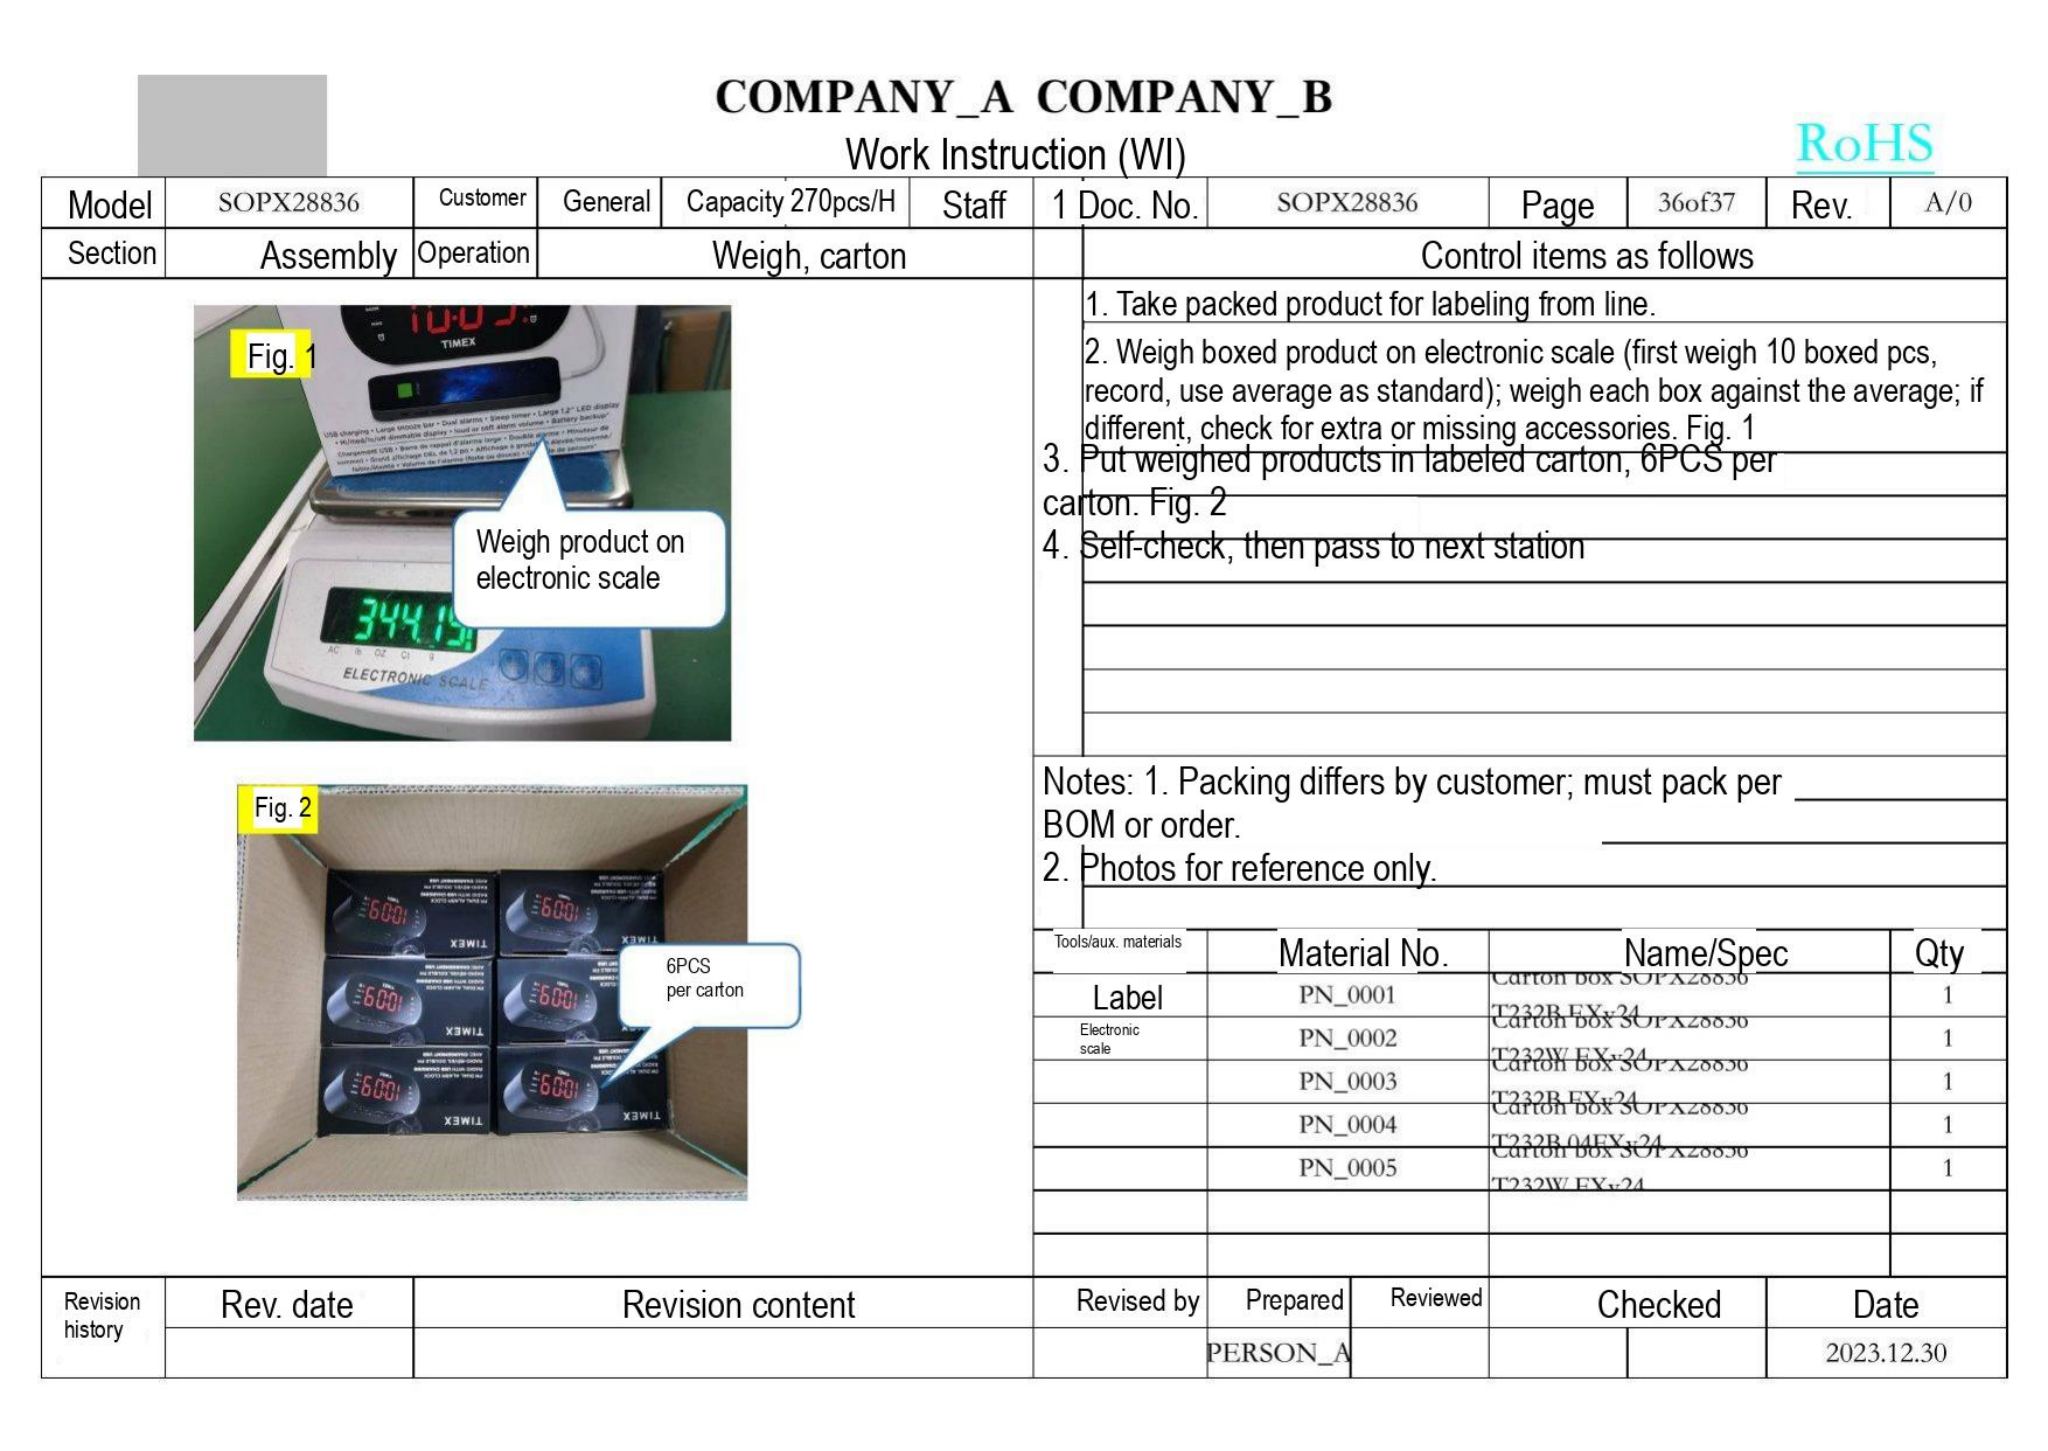# COMPANY_A COMPANY_B

Work Instruction (WI)

RoHS

| Model | SOPX28836 | Customer | General | Capacity 270pcs/H | Staff | 1 | Doc. No. | SOPX28836 | Page | 36of37 | Rev. | A/0 |
|---|---|---|---|---|---|---|---|---|---|---|---|---|
| Section | Assembly | Operation | Weigh, carton | | | | | | | | | |

Fig. 1

TIMEX

Weigh product on electronic scale

344.15

ELECTRONIC SCALE

Fig. 2

TIMEX

6:00

6PCS per carton

Control items as follows

1. Take packed product for labeling from line.
2. Weigh boxed product on electronic scale (first weigh 10 boxed pcs, record, use average as standard); weigh each box against the average; if different, check for extra or missing accessories. Fig. 1
3. Put weighed products in labeled carton, 6PCS per carton. Fig. 2
4. Self-check, then pass to next station

Notes: 1. Packing differs by customer; must pack per BOM or order.
2. Photos for reference only.

| Tools/aux. materials | Material No. | Name/Spec | Qty |
|---|---|---|---|
| Label | PN_0001 | Carton box SOPX28836 T232B EXx24 | 1 |
| Electronic scale | PN_0002 | Carton box SOPX28836 T232W EXx24 | 1 |
| | PN_0003 | Carton box SOPX28836 T232B EXx24 | 1 |
| | PN_0004 | Carton box SOPX28836 T232B 04EXx24 | 1 |
| | PN_0005 | Carton box SOPX28836 T232W EXx24 | 1 |

| Revision history | Rev. date | Revision content | Revised by | Prepared | Reviewed | Checked | Date |
|---|---|---|---|---|---|---|---|
| | | | | PERSON_A | | | 2023.12.30 |
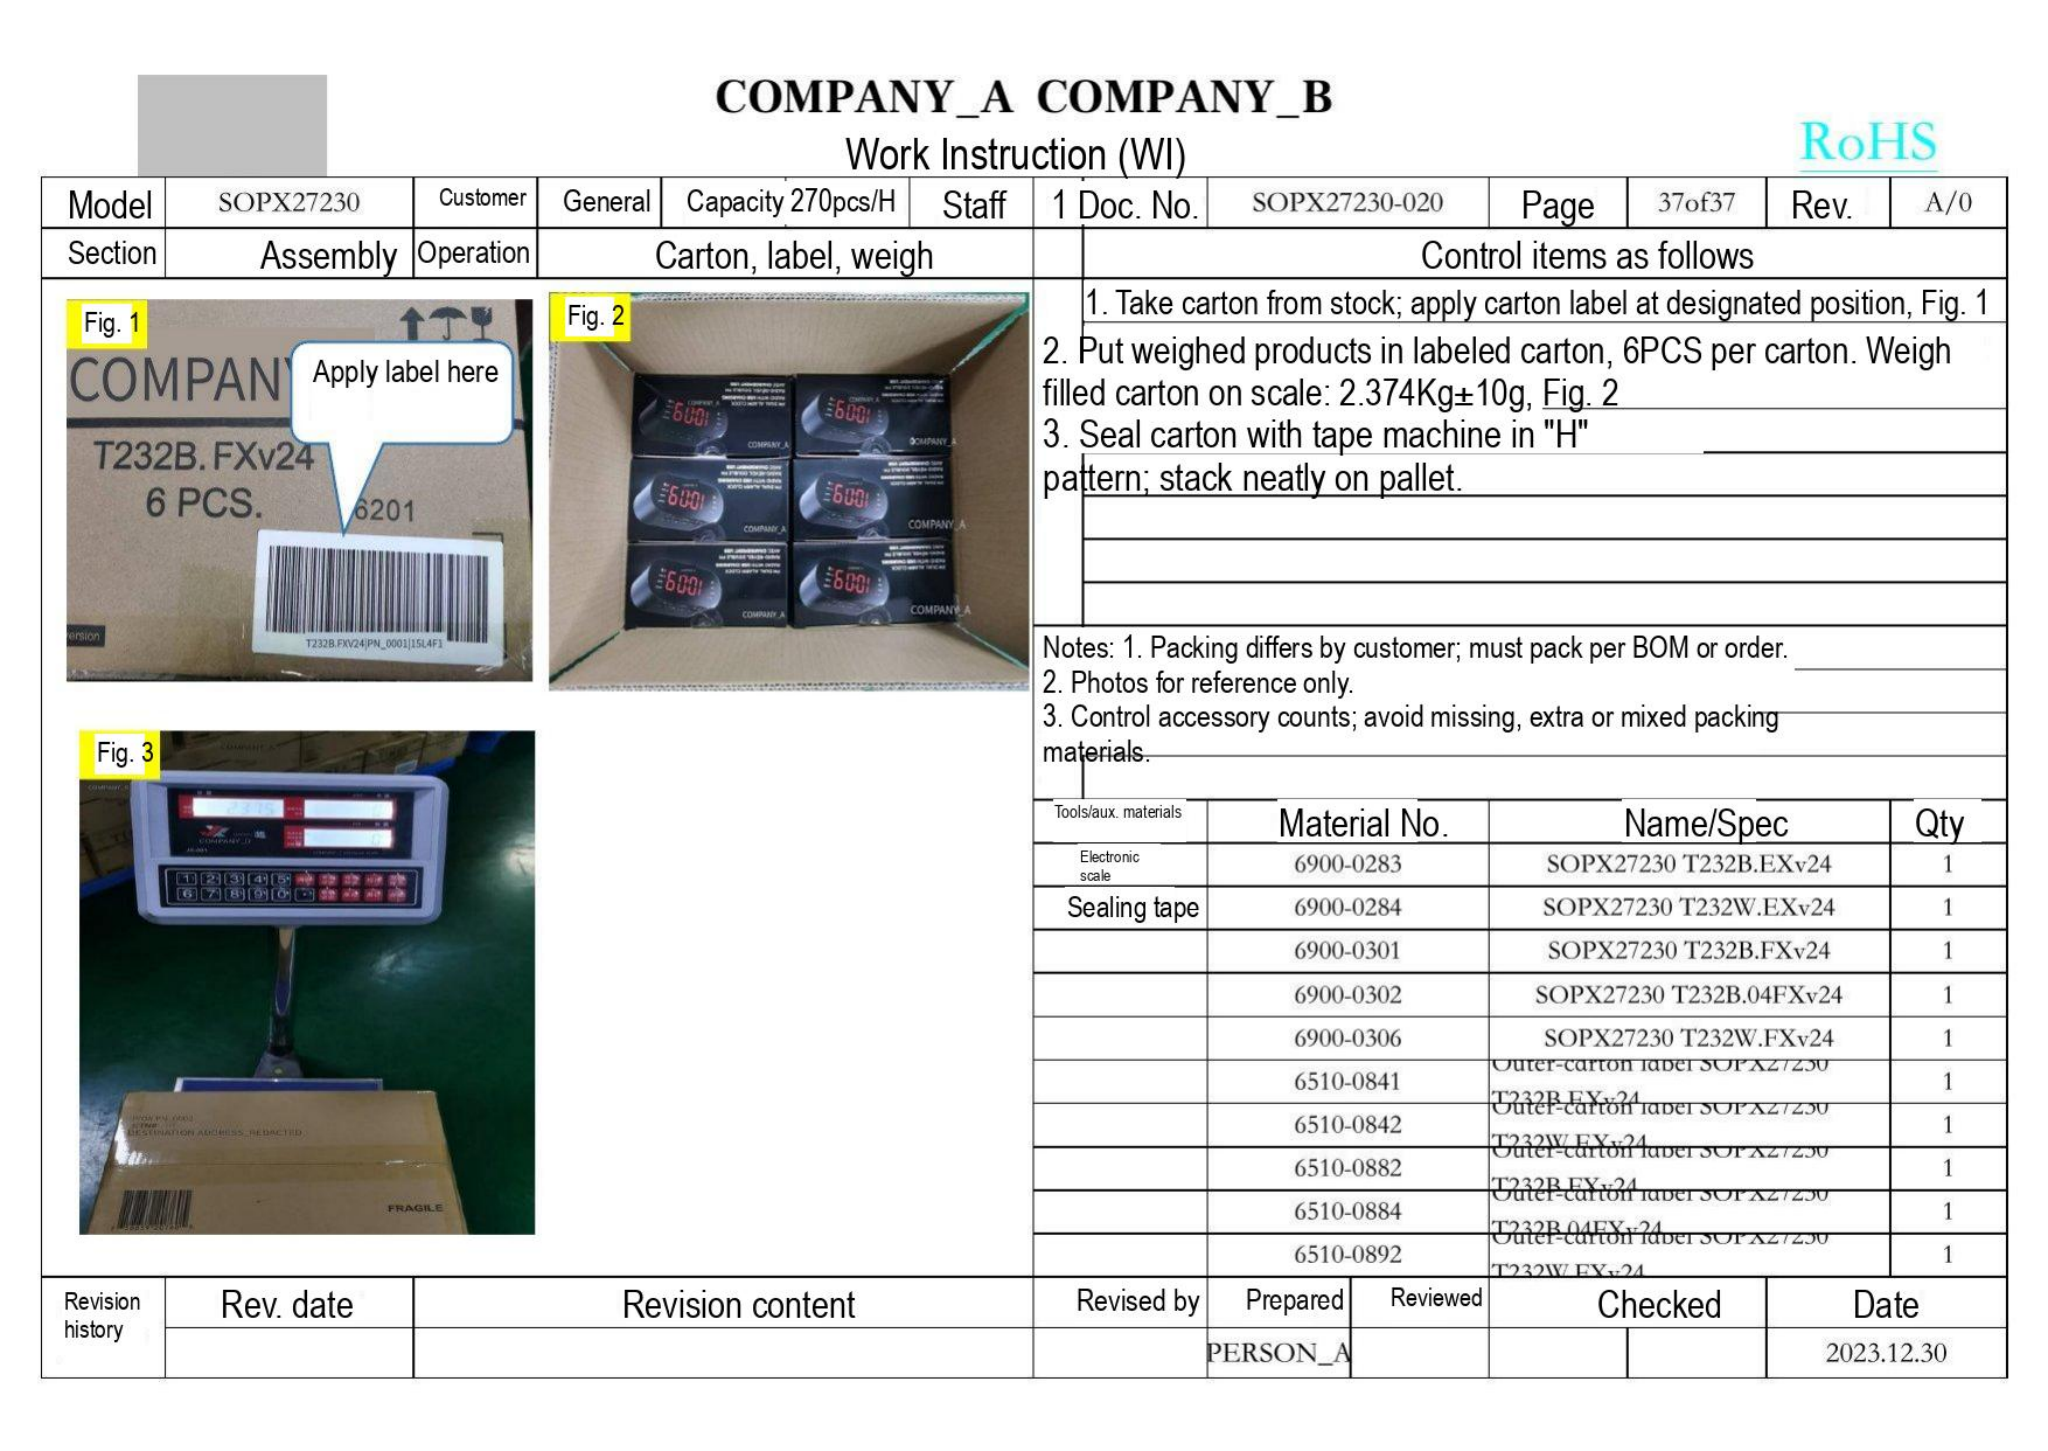# COMPANY_A COMPANY_B

Work Instruction (WI)

RoHS

| Model | SOPX27230 | Customer | General | Capacity 270pcs/H | Staff | 1 | Doc. No. | SOPX27230-020 | Page | 37of37 | Rev. | A/0 |
|---|---|---|---|---|---|---|---|---|---|---|---|---|
| Section | Assembly | Operation | Carton, label, weigh | | | | Control items as follows | | | | | |

Fig. 1

COMPAN

Apply label here

T232B.FXv24

6 PCS.

6201

T232B.FXV24|PN_0001|15L4F1

Fig. 2

COMPANY_A

Fig. 3

COMPANY_A

DESTINATION ADDRESS REDACTED

FRAGILE

1. Take carton from stock; apply carton label at designated position, Fig. 1
2. Put weighed products in labeled carton, 6PCS per carton. Weigh filled carton on scale: 2.374Kg±10g, Fig. 2
3. Seal carton with tape machine in "H" pattern; stack neatly on pallet.

Notes: 1. Packing differs by customer; must pack per BOM or order.
2. Photos for reference only.
3. Control accessory counts; avoid missing, extra or mixed packing materials.

| Tools/aux. materials | Material No. | Name/Spec | Qty |
|---|---|---|---|
| Electronic scale | 6900-0283 | SOPX27230 T232B.EXv24 | 1 |
| Sealing tape | 6900-0284 | SOPX27230 T232W.EXv24 | 1 |
| | 6900-0301 | SOPX27230 T232B.FXv24 | 1 |
| | 6900-0302 | SOPX27230 T232B.04FXv24 | 1 |
| | 6900-0306 | SOPX27230 T232W.FXv24 | 1 |
| | 6510-0841 | Outer-carton label SOPX27230 T232B.EXv24 | 1 |
| | 6510-0842 | Outer-carton label SOPX27230 T232W.EXv24 | 1 |
| | 6510-0882 | Outer-carton label SOPX27230 T232B.FXv24 | 1 |
| | 6510-0884 | Outer-carton label SOPX27230 T232B.04FXv24 | 1 |
| | 6510-0892 | Outer-carton label SOPX27230 T232W.FXv24 | 1 |

| Revision history | Rev. date | Revision content | Revised by | Prepared | Reviewed | Checked | Date |
|---|---|---|---|---|---|---|---|
| | | | | PERSON_A | | | 2023.12.30 |